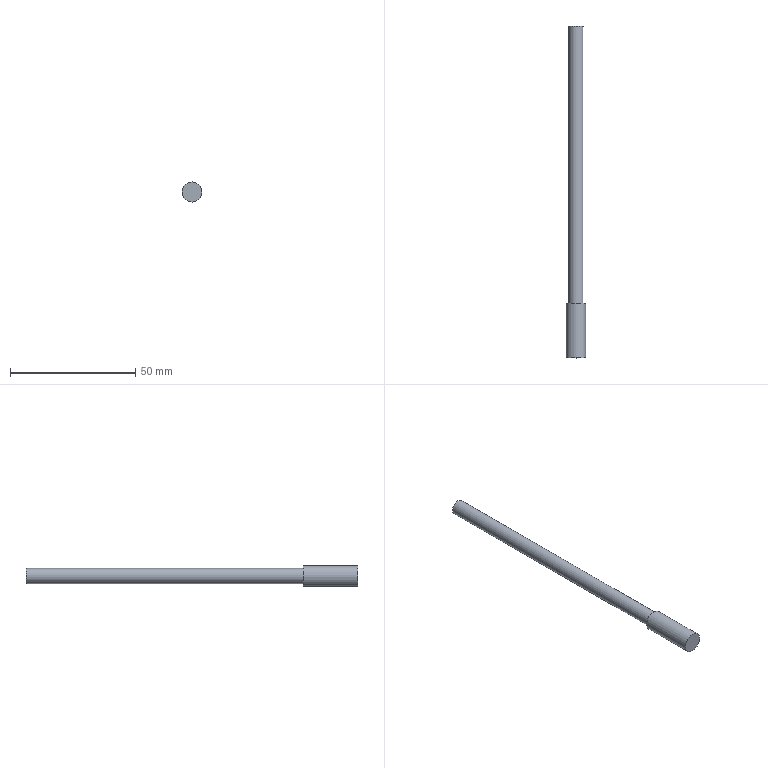Part | NX | features solid 2 | 1 solid | 5 faces | box 8 x 132.5 x 8 mm | volume 4228 mm3 | plane 3 | cylinder 2 | commonest cylinder face diameters 6 x1 8 x1
STEP:
#1=CARTESIAN_POINT('',(-67.,35.5,13.));
#2=VERTEX_POINT('',#1);
#3=CARTESIAN_POINT('',(-67.,35.5,10.));
#4=DIRECTION('',(0.,1.,0.));
#5=DIRECTION('',(0.,0.,1.));
#6=AXIS2_PLACEMENT_3D('',#3,#4,#5);
#7=CIRCLE('',#6,3.);
#8=EDGE_CURVE('',#2,#2,#7,.T.);
#9=ORIENTED_EDGE('',*,*,#8,.F.);
#10=EDGE_LOOP('',(#9));
#11=FACE_BOUND('',#10,.T.);
#12=CARTESIAN_POINT('',(-67.,-75.1,7.));
#13=VERTEX_POINT('',#12);
#14=CARTESIAN_POINT('',(-67.,-75.1,10.));
#15=DIRECTION('',(0.,1.,0.));
#16=DIRECTION('',(0.,0.,-1.));
#17=AXIS2_PLACEMENT_3D('',#14,#15,#16);
#18=CIRCLE('',#17,3.);
#19=EDGE_CURVE('',#13,#13,#18,.F.);
#20=ORIENTED_EDGE('',*,*,#19,.F.);
#21=EDGE_LOOP('',(#20));
#22=FACE_BOUND('',#21,.T.);
#23=CARTESIAN_POINT('',(-67.,-69.,10.));
#24=DIRECTION('',(0.,1.,0.));
#25=DIRECTION('',(-1.,0.,0.));
#26=AXIS2_PLACEMENT_3D('',#23,#24,#25);
#27=CYLINDRICAL_SURFACE('',#26,3.);
#28=ADVANCED_FACE('',(#11,#22),#27,.T.);
#29=ORIENTED_EDGE('',*,*,#8,.T.);
#30=EDGE_LOOP('',(#29));
#31=FACE_BOUND('',#30,.T.);
#32=CARTESIAN_POINT('',(-62.5,35.5,-5.));
#33=DIRECTION('',(0.,1.,0.));
#34=DIRECTION('',(0.,0.,1.));
#35=AXIS2_PLACEMENT_3D('',#32,#33,#34);
#36=PLANE('',#35);
#37=ADVANCED_FACE('',(#31),#36,.T.);
#38=CARTESIAN_POINT('',(-67.,-75.1,6.));
#39=VERTEX_POINT('',#38);
#40=CARTESIAN_POINT('',(-67.,-75.1,10.));
#41=DIRECTION('',(0.,1.,0.));
#42=DIRECTION('',(0.,0.,-1.));
#43=AXIS2_PLACEMENT_3D('',#40,#41,#42);
#44=CIRCLE('',#43,4.);
#45=EDGE_CURVE('',#39,#39,#44,.T.);
#46=ORIENTED_EDGE('',*,*,#45,.F.);
#47=EDGE_LOOP('',(#46));
#48=FACE_BOUND('',#47,.T.);
#49=CARTESIAN_POINT('',(-67.,-97.,6.));
#50=VERTEX_POINT('',#49);
#51=CARTESIAN_POINT('',(-67.,-97.,10.));
#52=DIRECTION('',(0.,1.,0.));
#53=DIRECTION('',(0.,0.,-1.));
#54=AXIS2_PLACEMENT_3D('',#51,#52,#53);
#55=CIRCLE('',#54,4.);
#56=EDGE_CURVE('',#50,#50,#55,.T.);
#57=ORIENTED_EDGE('',*,*,#56,.T.);
#58=EDGE_LOOP('',(#57));
#59=FACE_BOUND('',#58,.T.);
#60=CARTESIAN_POINT('',(-67.,-75.,10.));
#61=DIRECTION('',(0.,-1.,0.));
#62=DIRECTION('',(0.,0.,-1.));
#63=AXIS2_PLACEMENT_3D('',#60,#61,#62);
#64=CYLINDRICAL_SURFACE('',#63,4.);
#65=ADVANCED_FACE('',(#48,#59),#64,.T.);
#66=ORIENTED_EDGE('',*,*,#19,.T.);
#67=EDGE_LOOP('',(#66));
#68=FACE_BOUND('',#67,.T.);
#69=ORIENTED_EDGE('',*,*,#45,.T.);
#70=EDGE_LOOP('',(#69));
#71=FACE_BOUND('',#70,.T.);
#72=CARTESIAN_POINT('',(-67.,-75.1,10.));
#73=DIRECTION('',(0.,-1.,0.));
#74=DIRECTION('',(0.,0.,-1.));
#75=AXIS2_PLACEMENT_3D('',#72,#73,#74);
#76=PLANE('',#75);
#77=ADVANCED_FACE('',(#68,#71),#76,.F.);
#78=ORIENTED_EDGE('',*,*,#56,.F.);
#79=EDGE_LOOP('',(#78));
#80=FACE_BOUND('',#79,.T.);
#81=CARTESIAN_POINT('',(-62.5,-97.,-5.));
#82=DIRECTION('',(0.,-1.,0.));
#83=DIRECTION('',(0.,0.,1.));
#84=AXIS2_PLACEMENT_3D('',#81,#82,#83);
#85=PLANE('',#84);
#86=ADVANCED_FACE('',(#80),#85,.T.);
#87=CLOSED_SHELL('',(#28,#37,#65,#77,#86));
#88=MANIFOLD_SOLID_BREP('',#87);
#89=(LENGTH_UNIT()NAMED_UNIT(*)SI_UNIT(.MILLI.,.METRE.));
#90=UNCERTAINTY_MEASURE_WITH_UNIT(LENGTH_MEASURE(0.00001),#89,'','');
#91=(NAMED_UNIT(*)PLANE_ANGLE_UNIT()SI_UNIT($,.RADIAN.));
#92=(NAMED_UNIT(*)SI_UNIT($,.STERADIAN.)SOLID_ANGLE_UNIT());
#93=(GEOMETRIC_REPRESENTATION_CONTEXT(3)GLOBAL_UNCERTAINTY_ASSIGNED_CONTEXT((#90))GLOBAL_UNIT_ASSIGNED_CONTEXT((#89,#91,#92))REPRESENTATION_CONTEXT('',''));
#94=ADVANCED_BREP_SHAPE_REPRESENTATION('',(#88),#93);